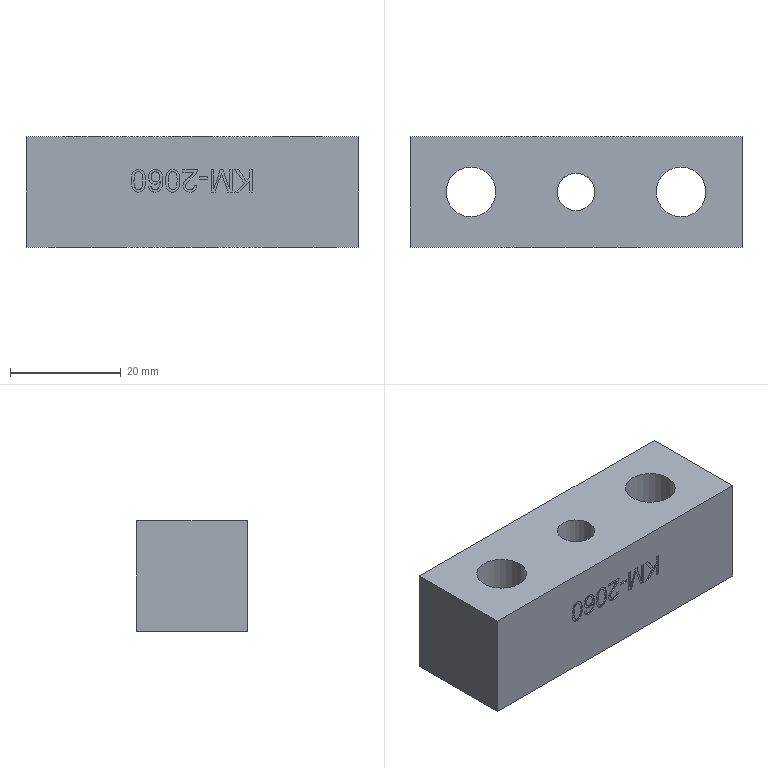Part | STEP file | lll_id742_x_t | 1 solid | 76 faces | box 60 x 20 x 20 mm | volume 18698 mm3 | plane 51 | other 19 | cylinder 6 | commonest cylinder face diameters 9 x3 14 x2 6.8 x1